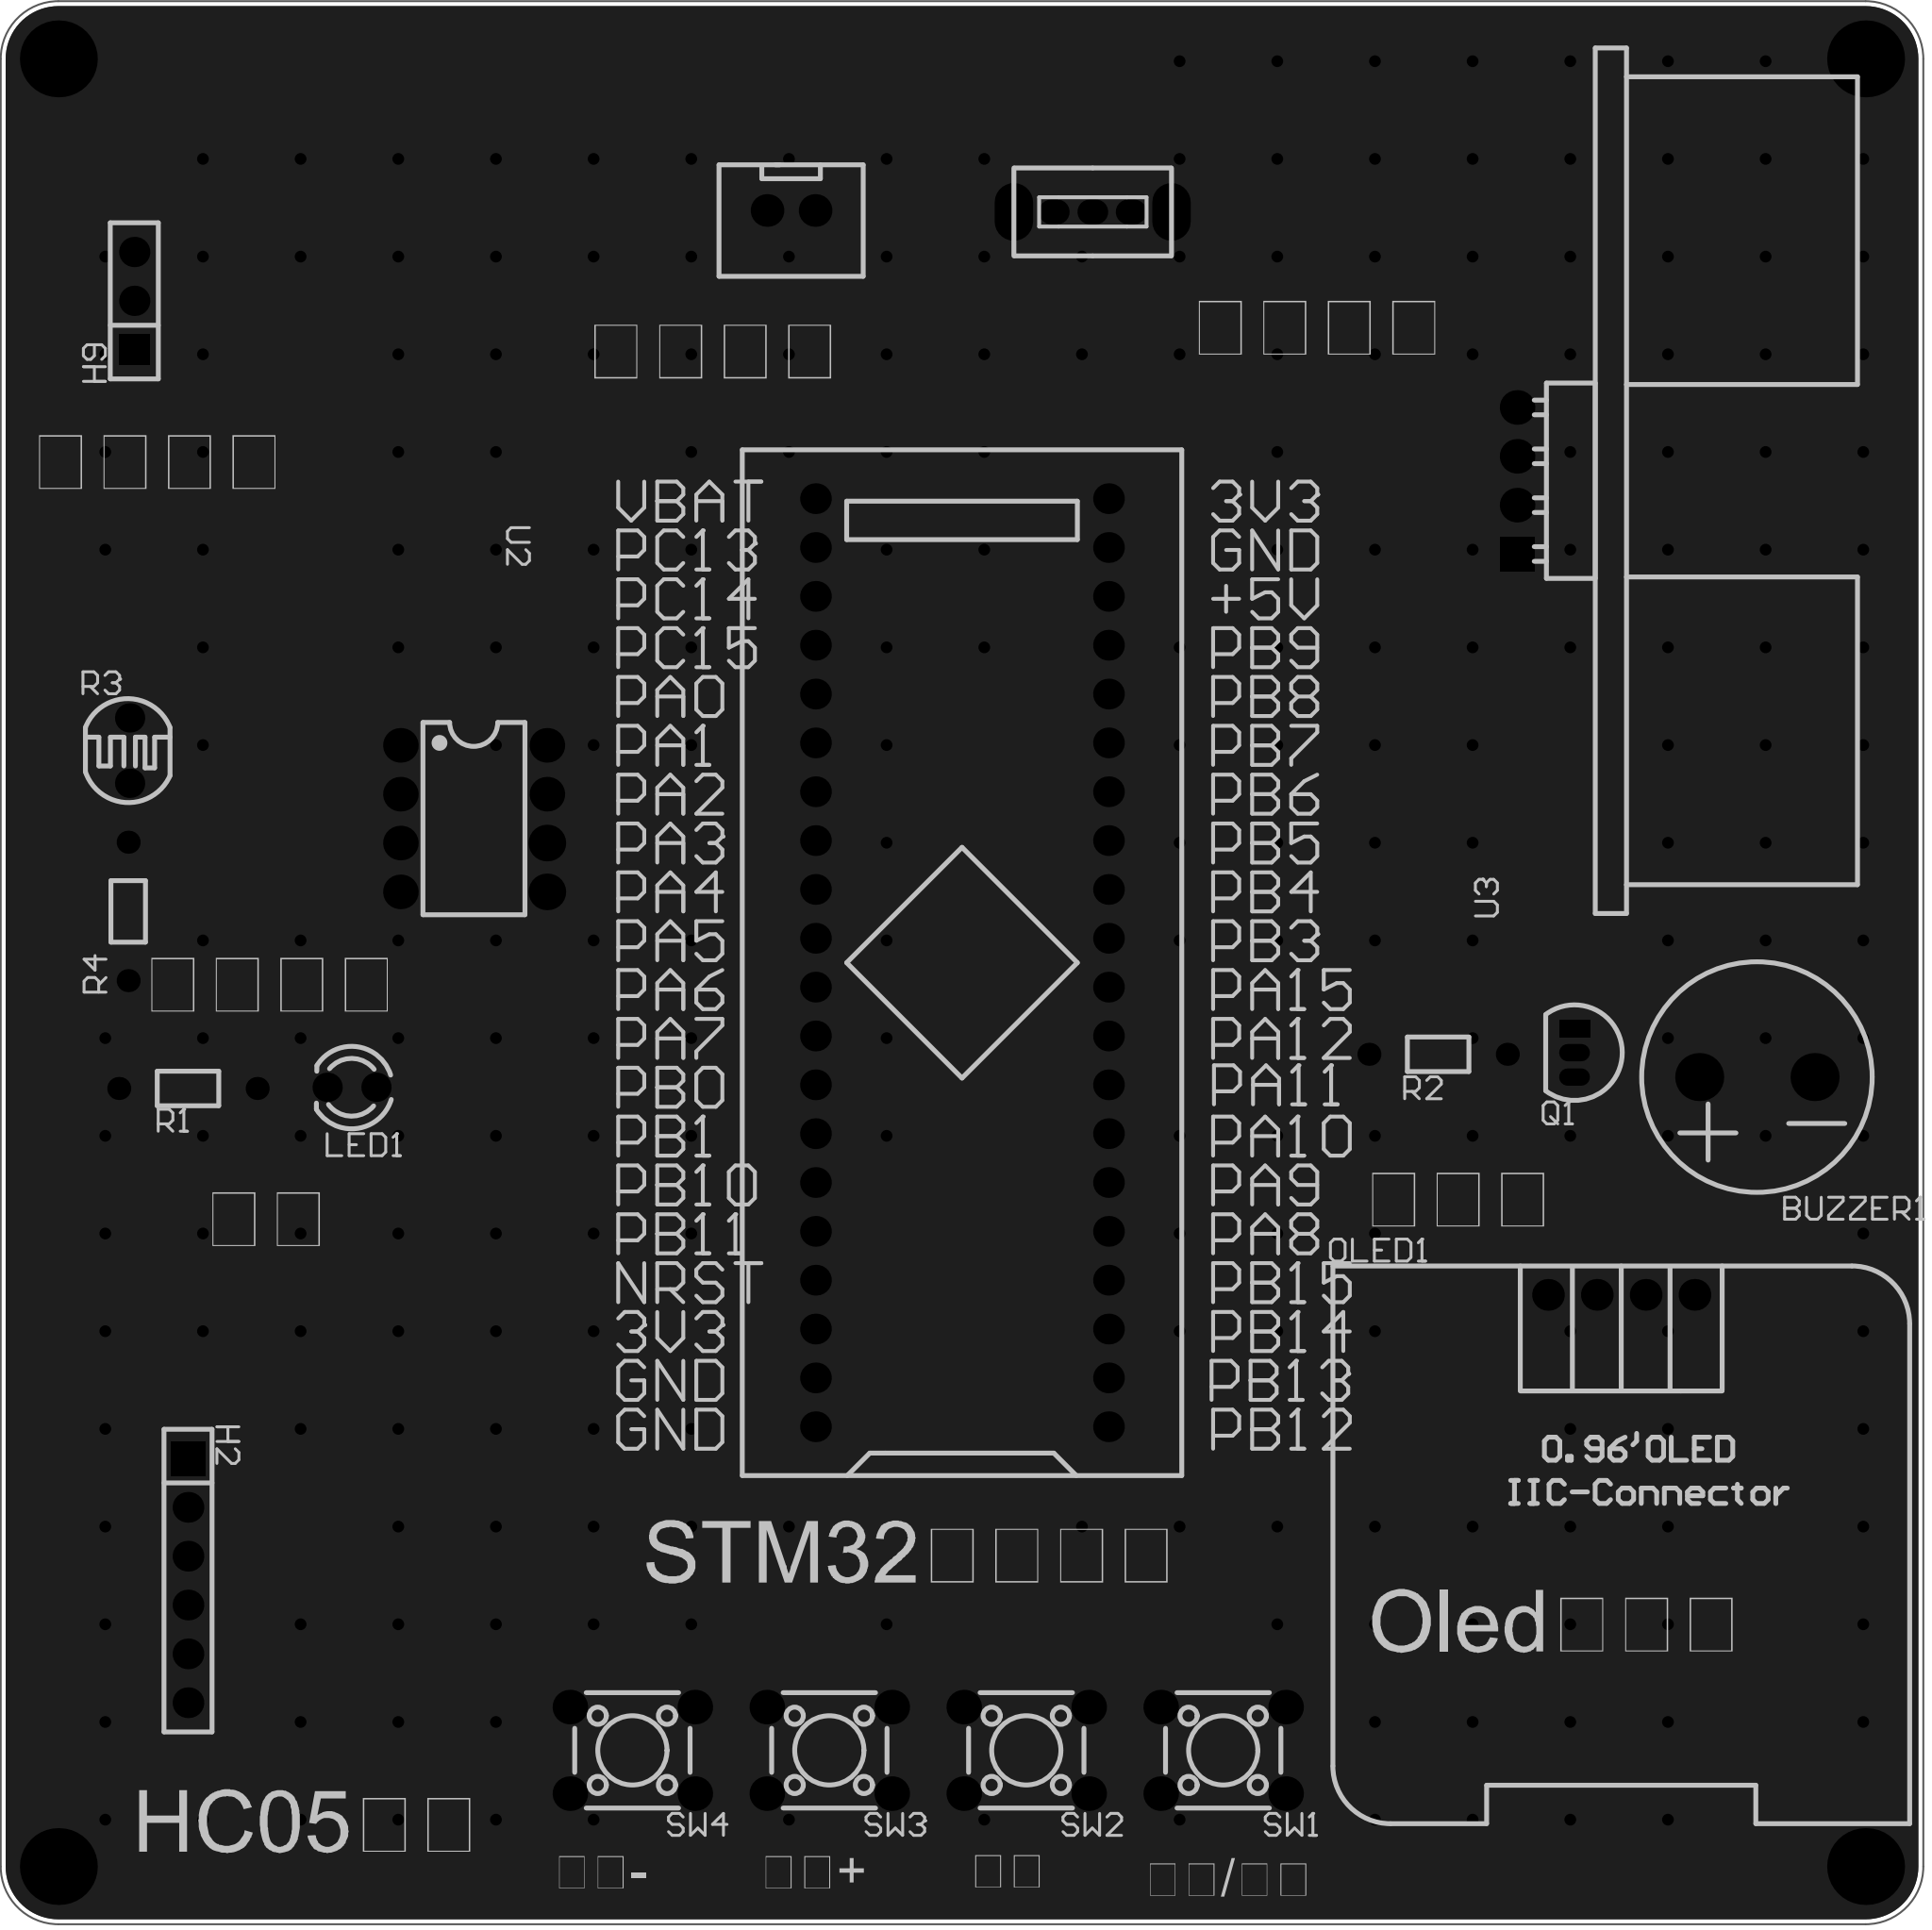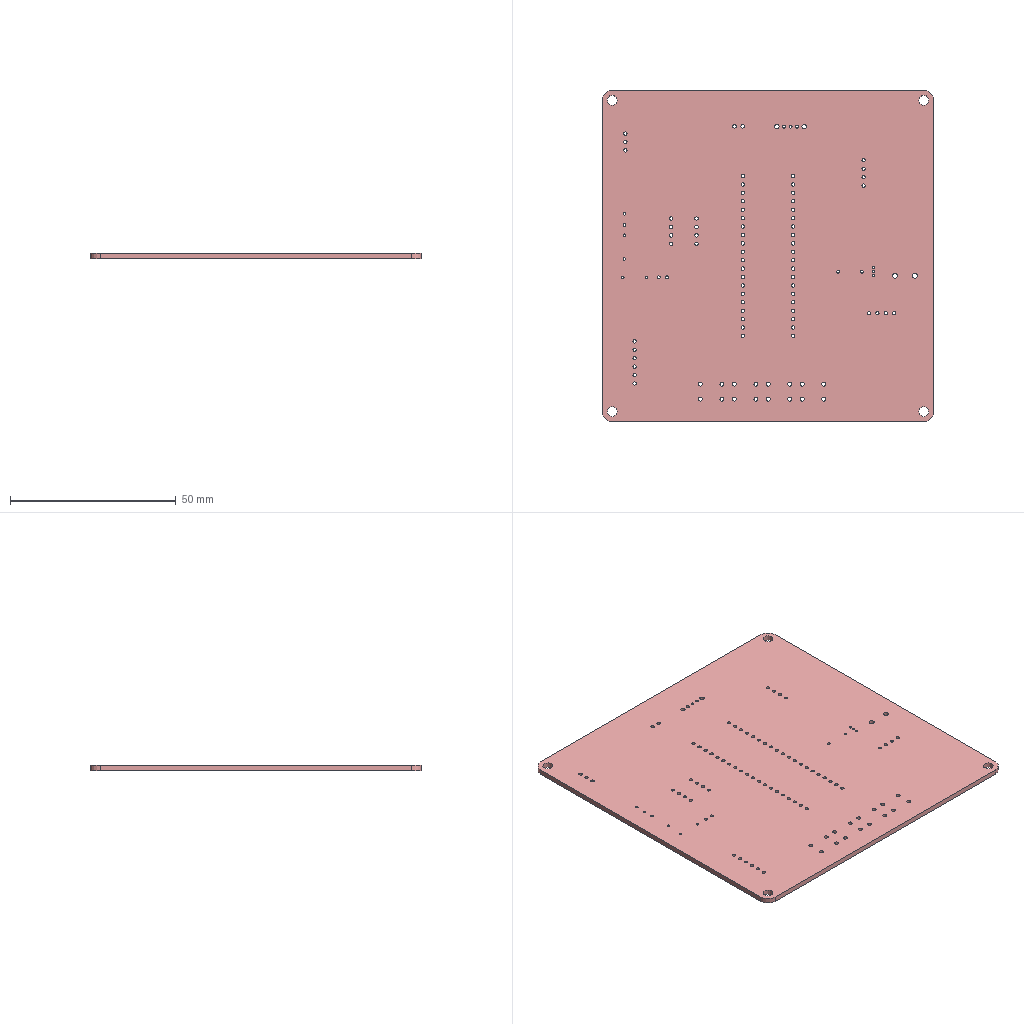Circuit board layout | Altium Designer | box 100 x 100 x 1.6 mm
Layer stack:
# Altium Designer layer stack of  (unit mm; dielectric type: 0 none, 1 core, 2 prepreg, 3 surface material)
index,name,kind,layer,copper_thickness_mm,dielectric_type,dielectric_thickness_mm,dielectric_material,dielectric_constant
0,Top Paste Mask Layer,other,,,,,,
1,Top Silkscreen Layer,other,,,,,,
2,Top Solder Mask Layer,dielectric,,,3,0.01,,3.3
3,Top Layer,copper,Top Layer,0.035,,,,
4,Dielectric1,dielectric,,,3,1.51,FR4,4.5
5,Bottom Layer,copper,Bottom Layer,0.035,,,,
6,Bottom Solder Mask Layer,dielectric,,,3,0.01,,3.3
7,Bottom Silkscreen Layer,other,,,,,,
8,Bottom Paste Mask Layer,other,,,,,,
# drill layer pairs: low layer,high layer
drill_pair,Top Layer,Bottom Layer
Part placement:
Designator,Comment,Layer,Footprint,Center-X(mm),Center-Y(mm),Rotation
U1,STM32F103C8T6-Card,TopLayer,CONN-TH_L53.3-W22.9_STM32F103C8T6-CARD,141.351,130.937,90
SW1,,TopLayer,SW-TH_4P-L6.0-W6.0-P4.50-LS6.5,154.936,89.979,180
SW2,,TopLayer,SW-TH_4P-L6.0-W6.0-P4.50-LS6.5,144.693,89.979,180
SW3,,TopLayer,SW-TH_4P-L6.0-W6.0-P4.50-LS6.5,134.449,89.979,180
SW4,,TopLayer,SW-TH_4P-L6.0-W6.0-P4.50-LS6.5,124.206,89.979,180
CN4,XH2.54*2P_直插,TopLayer,CONN-TH_2P-P2.50-XH2.54-2P,132.461,170.053,0
SW5,,TopLayer,拨动开关,148.148,169.978,180
H2,,TopLayer,HDR-TH_6P-P2.54-V-F,101.092,98.806,270
BUZZER1,buzzer,TopLayer,BUZ-TH_BD12.0-P6.00-D0.9-RD,182.697,124.99,180
LED1,,TopLayer,LED_TH-3mm,109.601,124.459,180
R1,100,TopLayer,Res_1/8W,101.092,124.397,180
H9,,TopLayer,HDR-TH_3P-P2.54-V-F,98.298,165.354,90
OLED1,,TopLayer,0.96OLED_4P,175.641,113.665,0
U2,ADC0832BCN,TopLayer,PDIP-8_L9.6-W6.4-P2.54-LS7.6-BL,115.951,138.43,270
R3,GL5549(80-100),TopLayer,RES-TH_L5.1-W4.3-P3.40-D0.5,98.057,141.966,0
R4,10kΩ,TopLayer,Res_1/8W,97.981,133.604,90
U3,HC-SR04,TopLayer,TH_HC-SR04V,170.224,156,90
Q1,,TopLayer,S8550P_TO-92,173.21,126.26,270
R2,1kΩ,TopLayer,Res_1/8W,166.116,126.175,180
Pad and via stacks:
# Altium Designer via and pad stacks of  (unit mm). Each distinct definition once, with the count of objects using it.
# via: kind,start_layer,end_layer,hole_mm,diameter_mm,mode(0 simple;1 top-mid-bottom;2 full stack),diameter_per_layer,count,example_net
# pad: kind,layer,hole_mm,hole_type(0 round;1 square;2 slot),plating,top_size,top_shape(1 round;2 rect;3 octagon;9 rounded rect),mid_size,bottom_size,mode,footprint,size_per_layer,count,example
pad,Multi-Layer,3,0,plated,4x4,1,4x4,4x4,0,,,4,1
pad,Multi-Layer,1,0,plated,1.6x1.6,1,1.6x1.6,1.6x1.6,0,CONN-TH_L53.3-W22.9_STM32F103C8T6-CARD,,40,U1.1
pad,Multi-Layer,1.2,0,plated,1.8x1.8,1,1.8x1.8,1.8x1.8,0,SW-TH_4P-L6.0-W6.0-P4.50-LS6.5,,16,SW1.1
pad,Multi-Layer,1.05,0,plated,1.7x1.7,1,1.7x1.7,1.7x1.7,0,CONN-TH_2P-P2.50-XH2.54-2P,,2,CN4.2
pad,Multi-Layer,0.8992,0,plated,1.6x1.3,1,1.6x1.3,1.6x1.3,0,\u00B2\u00A6\u00B6\u00AF\u00BF\u00AA\u00B9\u00D8,,3,SW5.1
pad,Multi-Layer,1.3,0,plated,3x1.999,1,3x1.999,3x1.999,0,\u00B2\u00A6\u00B6\u00AF\u00BF\u00AA\u00B9\u00D8,,2,SW5.4
pad,Multi-Layer,1.02,0,plated,1.6x1.6,1,1.6x1.6,1.6x1.6,0,HDR-TH_6P-P2.54-V-F,,5,H2.6
pad,Multi-Layer,1.02,0,plated,1.8x1.8,2,1.8x1.8,1.8x1.8,0,HDR-TH_6P-P2.54-V-F,,1,H2.1
pad,Multi-Layer,1.5,0,plated,2.5x2.5,1,2.5x2.5,2.5x2.5,0,BUZ-TH_BD12.0-P6.00-D0.9-RD,,2,BUZZER1.1
pad,Multi-Layer,0.9144,0,plated,1.524x1.524,1,1.524x1.524,1.524x1.524,0,LED_TH-3mm,,2,LED1.1
pad,Multi-Layer,0.8001,0,plated,1.199x1.199,1,1.199x1.199,1.199x1.199,0,Res_1/8W,,6,R1.1
pad,Multi-Layer,1.02,0,plated,1.575x1.575,1,1.575x1.575,1.575x1.575,0,HDR-TH_3P-P2.54-V-F,,2,H9.3
pad,Multi-Layer,1.02,0,plated,1.575x1.575,2,1.575x1.575,1.575x1.575,0,HDR-TH_3P-P2.54-V-F,,1,H9.1
pad,Multi-Layer,1,0,plated,1.65x1.65,1,1.65x1.65,1.65x1.65,0,0.96OLED_4P,,4,OLED1.4
pad,Multi-Layer,1,0,plated,1.8x1.8,1,1.8x1.8,1.8x1.8,0,PDIP-8_L9.6-W6.4-P2.54-LS7.6-BL,,6,U2.1
pad,Multi-Layer,1,0,plated,1.905x1.905,1,1.905x1.905,1.905x1.905,0,PDIP-8_L9.6-W6.4-P2.54-LS7.6-BL,,2,U2.5
pad,Multi-Layer,0.762,0,plated,1.524x1.524,1,1.524x1.524,1.524x1.524,0,RES-TH_L5.1-W4.3-P3.40-D0.5,,2,R3.2
pad,Multi-Layer,1.001,0,plated,1.8x1.8,1,1.8x1.8,1.8x1.8,0,TH_HC-SR04V,,3,U3.4
pad,Multi-Layer,1.001,0,plated,1.8x1.8,2,1.8x1.8,1.8x1.8,0,TH_HC-SR04V,,1,U3.1
pad,Multi-Layer,0.7,0,plated,0.9x1.6,1,0.9x1.6,0.9x1.6,0,S8550P_TO-92,,2,Q1.3
pad,Multi-Layer,0.7,0,plated,0.9x1.6,2,0.9x1.6,0.9x1.6,0,S8550P_TO-92,,1,Q1.1
via,Top Layer,Bottom Layer,0.3048,0.61,0,,247,GND
Copper pours:
name,layer,net,type(0 solid;1 hatched;2 none)
Bottom Layer-GND,Bottom Layer,GND,0
Top Layer-GND,Top Layer,GND,0
Design rules, without the lines most boards share:
# Altium Designer design rules of  (exported by Altium Designer, unit mm)
# columns: name | kind | enabled | priority | scope1 | scope2 | descriptor | typed fields (field=value)
Copper_copperRegion_copperThickness1oz | 0 | disabled | 4 | All | All | Clearance Constraint (Gap=5.984mil) (Disabled)(All),(All) | gap=0.152
Copper_copperRegion_copperThickness1oz_1 | 63 | disabled | 4 | All | All | Board Clearance Constraint (Gap=0mil) (Disabled)(All) |
Copper_copperRegion_Copper_copperRegion | 0 | disabled | 5 | All | All | Clearance Constraint (Gap=5.984mil) (Disabled)(All),(All) | gap=0.152
Copper_copperRegion_Copper_copperRegion_1 | 63 | disabled | 5 | All | All | Board Clearance Constraint (Gap=0mil) (Disabled)(All) |
copperThickness1oz | 0 | enabled | 6 | All | All | Clearance Constraint (Gap=5.984mil) (All),(All) | gap=0.152
copperThickness1oz_1 | 63 | enabled | 6 | All | All | Board Clearance Constraint (Gap=0mil) (All) |
copperRegion_copperThickness1oz | 20 | disabled | 1 | All | All | Polygon Connect Rule(Relief Connect )(Conductor Width=10mil) (Relief Angle=90 Angle) (Entries=4) (Air Gap Width=10mil) (Disabled)(All),(All) | connect_style(0=relief,1=direct,2=none)=0 relief_conductor_width=0.254 relief_entries=4
copperRegion_Copper_copperRegion | 20 | disabled | 2 | All | All | Polygon Connect Rule(Relief Connect )(Conductor Width=10mil) (Relief Angle=90 Angle) (Entries=4) (Air Gap Width=10mil) (Disabled)(All),(All) | connect_style(0=relief,1=direct,2=none)=0 relief_conductor_width=0.254 relief_entries=4
copperRegion | 20 | enabled | 3 | All | All | Polygon Connect Rule(Relief Connect )(Conductor Width=10mil) (Relief Angle=90 Angle) (Entries=4) (Air Gap Width=10mil) (All),(All) | connect_style(0=relief,1=direct,2=none)=0 relief_conductor_width=0.254 relief_entries=4